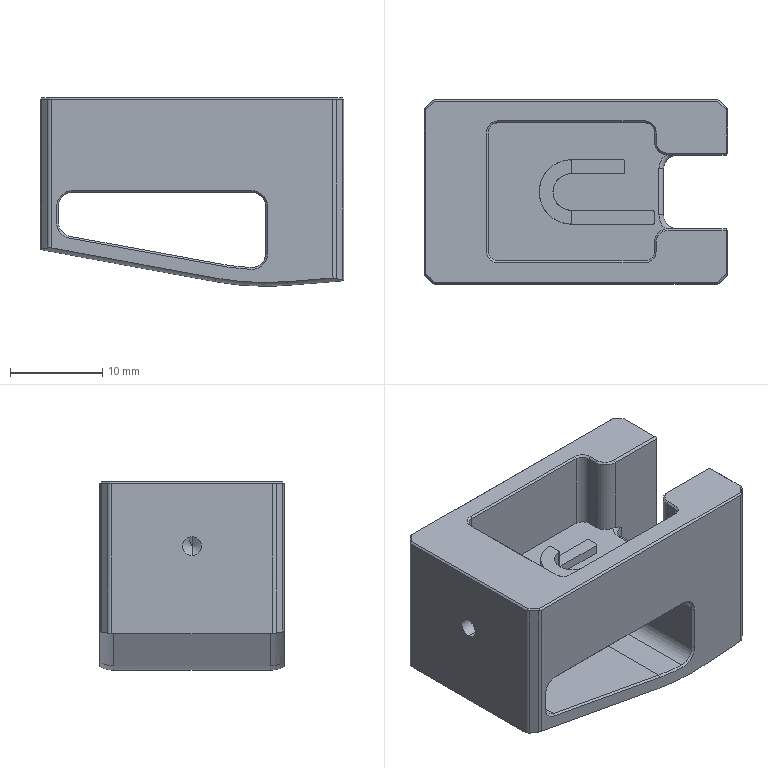NC program | NX | posted with a generic post | part box 33 x 20 x 20.478 mm
Lines 1 to 1476 of 8500:
N10 G17 G21 G94 G90
(FLOOR_WALL , TOOL : D80)
N12 T19 M6
N14 G54
N16 G17 G0 G90 X-64.5 Y0. B0. C0. S6500 M3
N18 G43 Z13. H19
N20 Z3.
N22 G94 G1 Z0. F1500.
N24 X-61.5
N26 X61.5
N28 X64.5
N30 Z3.
N32 G0 Z13.
N34 M5
(ADAPTIVE_MILLING , TOOL : D10)
N36 T15 M6
N38 G54
N40 G17 G0 G90 X-29.197 Y-0.049 B0. C0. S9500 M3
N42 G43 Z11. H15
N44 Z-17.478
N46 G94 G1 Z-20.478 F1000.
N48 X-27.84 Y-0.579 F3000.
N50 G3 X-26.55 Y-0.049 R1.015
N52 X-25.906 Y3.11 R9.424
N54 X-25.693 Y12.706 R184.544
N56 G2 X-22.784 Y17.042 R6.041
N58 X-17.015 Y18.852 R13.38
N60 X-8.025 Y19.178 R88.847
N62 G1 X-6.225 Y19.184
N64 X-3.525 Y19.188
N66 X2.075 Y19.19
N68 X18.775
N70 X18.875 Y19.189
N72 X18.975 Y19.186
N74 G2 X23.412 Y16.453 R5.88
N76 X25.313 Y10.821 R12.745
N78 X25.672 Y2.634 R73.061
N80 X25.665 Y-12.765 R826.306
N82 X22.794 Y-17.018 R6.043
N84 X17.429 Y-18.797 R12.91
N86 X8.943 Y-19.173 R72.366
N88 G1 X7.543 Y-19.18
N90 X5.643 Y-19.185
N92 X2.543 Y-19.189
N94 X-5.657 Y-19.19
N96 X-18.757
N98 X-18.857 Y-19.189
N100 G2 X-23.227 Y-16.711 R5.739
N102 X-25.255 Y-11.235 R12.019
N104 X-25.571 Y-1.555 R52.678
N106 G3 X-24.923 Y10.121 R113.262
N108 G2 X-21.008 Y16.066 R7.723
N110 X-14.843 Y17.969 R15.574
N112 X-5.557 Y18.363 R84.404
N114 G1 X-4.057 Y18.37
N116 X-2.057 Y18.376
N118 X1.043 Y18.38
N120 X8.043 Y18.381
N122 X16.043 Y18.382
N124 X16.143 Y18.381
N126 G2 X22.423 Y14.693 R7.557
N128 X24.435 Y8.568 R14.865
N130 X24.862 Y-0.917 R80.933
N132 X24.843 Y-10.316 R246.554
N134 X20.874 Y-16.119 R7.736
N136 X14.498 Y-18.009 R16.025
N138 X4.809 Y-18.367 R97.281
N140 G1 X3.209 Y-18.373
N142 X0.909 Y-18.378
N144 X-3.191 Y-18.381
N146 X-15.991 Y-18.382
N148 X-16.191 Y-18.38
N150 X-16.391 Y-18.373
N152 G2 X-22.556 Y-14.484 R7.647
N154 X-24.481 Y-8.223 R15.541
N156 X-24.519 Y0.46 R41.857
N158 G3 X-24.138 Y8.349 R857.805
N160 G2 X-19.144 Y15.38 R8.958
N162 X-12.327 Y17.203 R18.779
N164 X-2.337 Y17.556 R111.284
N166 X14.563 Y17.545 R890.638
N168 X21.801 Y12.722 R8.805
N170 X23.698 Y5.825 R18.339
N172 X24.062 Y-5.465 R122.093
N174 X23.845 Y-9.449 R18.233
N176 X18.864 Y-15.488 R9.011
N178 X12.221 Y-17.21 R19.143
N180 X1.331 Y-17.561 R120.966
N182 X-14.568 Y-17.544 R863.034
N184 X-21.805 Y-12.718 R8.797
N186 X-23.724 Y-5.018 R18.167
N188 X-23.56 Y3.077 R99.096
N190 X-23.222 Y7.659 R30.846
N192 X-17.67 Y14.575 R9.873
N194 X-10.537 Y16.389 R20.72
N196 X0.553 Y16.75 R125.976
N198 X12.853 Y16.726 R517.693
N200 X20.669 Y11.829 R9.524
N202 X22.219 Y7.985 R12.151
N204 X23.154 Y-0.347 R39.823
N206 X23.165 Y-6.844 R65.853
N208 X18.349 Y-14.153 R9.47
N210 X14.968 Y-15.59 R11.098
N212 X7.053 Y-16.624 R34.899
N214 X-12.745 Y-16.731 R554.895
N216 X-20.659 Y-11.841 R9.502
N218 X-22.178 Y-8.076 R11.391
N220 X-22.815 Y-0.424 R30.38
N222 X-22.52 Y5.764 R52.429
N224 X-21.597 Y8.818 R12.776
N226 X-20.808 Y11.647 R6.481
N228 X-18.029 Y14.376 R9.736
N230 X-15.327 Y15.096 R6.531
N232 X0.91 Y15.934 R136.055
N234 X11.409 Y15.9 R258.588
N236 X14.907 Y15.115 R12.167
N238 X16.806 Y14.883 R27.804
N240 X19.277 Y13.435 R6.592
N242 X20.711 Y11.773 R10.839
N244 G1 X20.808 Y11.647
N246 X20.876 Y11.529
N248 G2 X21.596 Y8.827 R6.531
N250 X22.374 Y-4.51 R121.46
N252 X21.618 Y-8.318 R11.799
N254 X21.383 Y-10.306 R19.905
N256 X19.935 Y-12.777 R6.592
N258 X18.273 Y-14.211 R10.839
N260 G3 X19.308 Y-15.909 R1.
N262 G1 X19.425 Y-15.854
N264 X21.234 Y-15.002 Z-20.378
N266 X22.493 Y-14.409
N268 X22.639 Y-14.319
N270 X22.773 Y-14.211
N272 X23.379 Y-13.588
N274 G3 X23.822 Y-12.725 R2.463
N276 X25.265 Y-5.267 R39.856
N278 G1 X25.37 Y-3.775
N280 X25.419 Y-2.28
N282 X25.497 Y6.509
N284 G3 X25.26 Y7.164 R1.032
N286 G1 X24.116 Y8.515
N288 X23.69 Y9.027 Z-20.412
N290 X23.245 Y9.522 Z-20.445
N292 G3 X22.634 Y9.758 Z-20.478 R1.04
N294 X21.6 Y8.759 R1.004
N296 G2 X21.535 Y1.067 R447.921
N298 X21.519 Y-3.583 R98.353
N300 G1 X21.596 Y-4.166
N302 X21.6 Y-4.234
N304 Y-8.534
N306 G3 X22.702 Y-9.632 R1.1
N308 X23.8 Y-8.533 R1.1
N310 G1 X23.786 Y4.024
N312 G3 X21.596 Y4.166 R1.1
N314 G2 X21.143 Y1.748 R17.605
N316 G3 X20.89 Y-1.537 R20.735
N318 G1 X20.913 Y-1.634
N320 X20.918 Y-1.67
N322 X20.943 Y-1.714
N324 X21.4 Y-2.816
N326 X21.435 Y-2.948
N328 X21.527 Y-3.642
N330 G3 X23.717 Y-3.461 R1.1
N332 G1 X23.516 Y2.433
N334 G3 X21.4 Y2.816 R1.1
N336 X20.425 Y-0.517 R9.925
N338 X20.875 Y-1.595 R1.48
N340 G1 X20.925 Y-1.682
N342 G3 X22.977 Y-1.141 R1.101
N344 G1 X22.996 Y1.155
N346 G3 X20.943 Y1.714 R1.101
N348 X20.145 Y-0.426 R3.301
N350 X20.619 Y-1.262 R1.968
N352 X22.586 Y-0.7 R1.101
N354 G1 X22.668 Y0.067
N356 X22.724 Y0.836
N358 G3 X20.753 Y1.437 R1.101
N360 X19.968 Y0.068 R3.065
N362 X20.324 Y-0.877 R1.267
N364 X22.281 Y-0.024 R1.101
N366 G1 X22.221 Y0.325
N368 X22.104 Y0.659
N370 G3 X20.266 Y0.802 R1.102
N372 X20.126 Y-0.615 R1.104
N374 G2 X21.435 Y-2.948 R5.91
N376 G1 X21.6 Y-4.234
N378 X21.596 Y-8.827
N380 G2 X20.808 Y-11.647 R6.449
N382 X18.029 Y-14.376 R9.847
N384 X15.327 Y-15.096 R6.531
N386 X-0.51 Y-15.932 R134.597
N388 X-11.409 Y-15.899 R272.221
N390 X-14.908 Y-15.115 R12.161
N392 X-16.806 Y-14.883 R28.628
N394 X-19.277 Y-13.435 R6.592
N396 X-20.711 Y-11.773 R10.839
N398 G3 X-22.409 Y-12.808 R1.
N400 G1 X-22.354 Y-12.925
N402 X-21.502 Y-14.734 Z-20.378
N404 X-20.909 Y-15.993
N406 X-20.819 Y-16.139
N408 X-20.711 Y-16.273
N410 X-20.088 Y-16.878
N412 G3 X-19.222 Y-17.311 R2.374
N414 G1 X-15.893 Y-18.146
N416 G3 X-9.41 Y-18.924 R30.044
N418 G1 X13.009 Y-18.997
N420 G3 X13.657 Y-18.761 R1.033
N422 G1 X15.013 Y-17.616
N424 X15.525 Y-17.19 Z-20.412
N426 X16.022 Y-16.746 Z-20.445
N428 G3 X16.258 Y-16.135 Z-20.478 R1.04
N430 X15.259 Y-15.1 R1.004
N432 G1 X-15.041
N434 G2 X-18.147 Y-14.308 R6.417
N436 X-20.876 Y-11.529 R9.847
N438 X-21.6 Y-8.759 R6.592
N440 X-21.824 Y3.627 R80.534
N442 G1 X-21.803 Y3.825
N444 X-21.779 Y4.024
N446 X-21.752 Y4.222
N448 X-21.738 Y4.321
N450 X-21.707 Y4.519
N452 X-21.655 Y4.814
N454 X-21.619 Y5.011
N456 X-21.603 Y5.11
N458 X-21.6 Y5.134
N460 Y8.759
N462 X-21.596 Y8.827
N464 G3 X-23.793 Y8.899 R-1.1
N466 G1 X-23.8 Y-8.758
N468 G3 X-22.699 Y-9.857 R1.1
N470 X-21.6 Y-8.759 R1.1
N472 G1 Y5.141
N474 X-21.596 Y8.827
N476 G2 X-20.808 Y11.647 R6.449
N478 X-18.029 Y14.376 R9.847
N480 G1 X-16.806 Y14.883
N482 X-16.674 Y14.918
N484 X-15.259 Y15.1
N486 X15.041
N488 G3 X16.011 Y15.828 R1.017
N490 G1 X16.487 Y17.463
N492 Z-17.478
N494 G0 Z11.
N496 M5
(ZLEVEL_PROFILE , TOOL : D6)
N498 T12 M6
N500 G54
N502 G17 G0 G90 X19.81 Y1.615 B0. C0. S9500 M3
N504 G43 Z30. H12
N506 Z0.001
N508 G94 G1 Z-0.499 F1800.
N510 X18.903 Y1.906
N512 G3 X18.317 Y1.779 R0.6
N514 G2 X16.3 Y1. R3.
N516 G1 X12.5
N518 Y-1.
N520 X16.3
N522 G2 X18.317 Y-1.779 R3.
N524 G3 X18.903 Y-1.906 R0.6
N526 G1 X19.81 Y-1.615
N528 Z0.001
N530 G0 Y1.615 Z-0.499
N532 G1 Z-0.999
N534 X18.903 Y1.906
N536 G3 X18.317 Y1.779 R0.6
N538 G2 X16.3 Y1. R3.
N540 G1 X12.5
N542 Y-1.
N544 X16.3
N546 G2 X18.317 Y-1.779 R3.
N548 G3 X18.903 Y-1.906 R0.6
N550 G1 X19.81 Y-1.615
N552 Z-0.499
N554 G0 Y1.615 Z-0.998
N556 G1 Z-1.498
N558 X18.903 Y1.906
N560 G3 X18.317 Y1.779 R0.6
N562 G2 X16.3 Y1. R3.
N564 G1 X12.5
N566 Y-1.
N568 X16.3
N570 G2 X18.317 Y-1.779 R3.
N572 G3 X18.903 Y-1.906 R0.6
N574 G1 X19.81 Y-1.615
N576 Z-0.998
N578 G0 Y1.615 Z-1.498
N580 G1 Z-1.998
N582 X18.903 Y1.906
N584 G3 X18.317 Y1.779 R0.6
N586 G2 X16.3 Y1. R3.
N588 G1 X12.5
N590 Y-1.
N592 X16.3
N594 G2 X18.317 Y-1.779 R3.
N596 G3 X18.903 Y-1.906 R0.6
N598 G1 X19.81 Y-1.615
N600 Z-1.498
N602 G0 Y1.615 Z-1.997
N604 G1 Z-2.497
N606 X18.903 Y1.906
N608 G3 X18.317 Y1.779 R0.6
N610 G2 X16.3 Y1. R3.
N612 G1 X12.5
N614 Y-1.
N616 X16.3
N618 G2 X18.317 Y-1.779 R3.
N620 G3 X18.903 Y-1.906 R0.6
N622 G1 X19.81 Y-1.615
N624 Z-1.997
N626 G0 Y1.615 Z-2.497
N628 G1 Z-2.997
N630 X18.903 Y1.906
N632 G3 X18.317 Y1.779 R0.6
N634 G2 X16.3 Y1. R3.
N636 G1 X12.5
N638 Y-1.
N640 X16.3
N642 G2 X18.317 Y-1.779 R3.
N644 G3 X18.903 Y-1.906 R0.6
N646 G1 X19.81 Y-1.615
N648 Z-2.497
N650 G0 Y1.615 Z-2.996
N652 G1 Z-3.496
N654 X18.903 Y1.906
N656 G3 X18.317 Y1.779 R0.6
N658 G2 X16.3 Y1. R3.
N660 G1 X12.5
N662 Y-1.
N664 X16.3
N666 G2 X18.317 Y-1.779 R3.
N668 G3 X18.903 Y-1.906 R0.6
N670 G1 X19.81 Y-1.615
N672 Z-2.996
N674 G0 Y1.615 Z-3.496
N676 G1 Z-3.996
N678 X18.903 Y1.906
N680 G3 X18.317 Y1.779 R0.6
N682 G2 X16.3 Y1. R3.
N684 G1 X12.5
N686 Y-1.
N688 X16.3
N690 G2 X18.317 Y-1.779 R3.
N692 G3 X18.903 Y-1.906 R0.6
N694 G1 X19.81 Y-1.615
N696 Z-3.496
N698 G0 Y1.615 Z-3.995
N700 G1 Z-4.495
N702 X18.903 Y1.906
N704 G3 X18.317 Y1.779 R0.6
N706 G2 X16.3 Y1. R3.
N708 G1 X12.5
N710 Y-1.
N712 X16.3
N714 G2 X18.317 Y-1.779 R3.
N716 G3 X18.903 Y-1.906 R0.6
N718 G1 X19.81 Y-1.615
N720 Z-3.995
N722 G0 Y1.615 Z-4.495
N724 G1 Z-4.995
N726 X18.903 Y1.906
N728 G3 X18.317 Y1.779 R0.6
N730 G2 X16.3 Y1. R3.
N732 G1 X12.5
N734 Y-1.
N736 X16.3
N738 G2 X18.317 Y-1.779 R3.
N740 G3 X18.903 Y-1.906 R0.6
N742 G1 X19.81 Y-1.615
N744 Z-4.495
N746 G0 Y1.615 Z-4.994
N748 G1 Z-5.494
N750 X18.903 Y1.906
N752 G3 X18.317 Y1.779 R0.6
N754 G2 X16.3 Y1. R3.
N756 G1 X12.5
N758 Y-1.
N760 X16.3
N762 G2 X18.317 Y-1.779 R3.
N764 G3 X18.903 Y-1.906 R0.6
N766 G1 X19.81 Y-1.615
N768 Z-4.994
N770 G0 Y1.615 Z-5.494
N772 G1 Z-5.994
N774 X18.903 Y1.906
N776 G3 X18.317 Y1.779 R0.6
N778 G2 X16.3 Y1. R3.
N780 G1 X12.5
N782 Y-1.
N784 X16.3
N786 G2 X18.317 Y-1.779 R3.
N788 G3 X18.903 Y-1.906 R0.6
N790 G1 X19.81 Y-1.615
N792 Z-5.494
N794 G0 Y1.615 Z-5.993
N796 G1 Z-6.493
N798 X18.903 Y1.906
N800 G3 X18.317 Y1.779 R0.6
N802 G2 X16.3 Y1. R3.
N804 G1 X12.5
N806 Y-1.
N808 X16.3
N810 G2 X18.317 Y-1.779 R3.
N812 G3 X18.903 Y-1.906 R0.6
N814 G1 X19.81 Y-1.615
N816 Z-5.993
N818 G0 Y1.615 Z-6.493
N820 G1 Z-6.993
N822 X18.903 Y1.906
N824 G3 X18.317 Y1.779 R0.6
N826 G2 X16.3 Y1. R3.
N828 G1 X12.5
N830 Y-1.
N832 X16.3
N834 G2 X18.317 Y-1.779 R3.
N836 G3 X18.903 Y-1.906 R0.6
N838 G1 X19.81 Y-1.615
N840 Z-6.493
N842 G0 Y1.615 Z-6.992
N844 G1 Z-7.492
N846 X18.903 Y1.906
N848 G3 X18.317 Y1.779 R0.6
N850 G2 X16.3 Y1. R3.
N852 G1 X12.5
N854 Y-1.
N856 X16.3
N858 G2 X18.317 Y-1.779 R3.
N860 G3 X18.903 Y-1.906 R0.6
N862 G1 X19.81 Y-1.615
N864 Z-6.992
N866 G0 Y1.615 Z-7.492
N868 G1 Z-7.992
N870 X18.903 Y1.906
N872 G3 X18.317 Y1.779 R0.6
N874 G2 X16.3 Y1. R3.
N876 G1 X12.5
N878 Y-1.
N880 X16.3
N882 G2 X18.317 Y-1.779 R3.
N884 G3 X18.903 Y-1.906 R0.6
N886 G1 X19.81 Y-1.615
N888 Z-7.492
N890 G0 Y1.615 Z-7.991
N892 G1 Z-8.491
N894 X18.903 Y1.906
N896 G3 X18.317 Y1.779 R0.6
N898 G2 X16.3 Y1. R3.
N900 G1 X12.5
N902 Y-1.
N904 X16.3
N906 G2 X18.317 Y-1.779 R3.
N908 G3 X18.903 Y-1.906 R0.6
N910 G1 X19.81 Y-1.615
N912 Z-7.991
N914 G0 Y1.615 Z-8.49
N916 G1 Z-8.99
N918 X18.903 Y1.906
N920 G3 X18.317 Y1.779 R0.6
N922 G2 X16.3 Y1. R3.
N924 G1 X12.5
N926 Y-1.
N928 X16.3
N930 G2 X18.317 Y-1.779 R3.
N932 G3 X18.903 Y-1.906 R0.6
N934 G1 X19.81 Y-1.615
N936 Z-8.49
N938 G0 Y1.615 Z-8.99
N940 G1 Z-9.49
N942 X18.903 Y1.906
N944 G3 X18.317 Y1.779 R0.6
N946 G2 X16.3 Y1. R3.
N948 G1 X12.5
N950 Y-1.
N952 X16.3
N954 G2 X18.317 Y-1.779 R3.
N956 G3 X18.903 Y-1.906 R0.6
N958 G1 X19.81 Y-1.615
N960 Z-8.99
N962 G0 Y1.615 Z-9.489
N964 G1 Z-9.989
N966 X18.903 Y1.906
N968 G3 X18.317 Y1.779 R0.6
N970 G2 X16.3 Y1. R3.
N972 G1 X12.5
N974 Y-1.
N976 X16.3
N978 G2 X18.317 Y-1.779 R3.
N980 G3 X18.903 Y-1.906 R0.6
N982 G1 X19.81 Y-1.615
N984 Z-9.489
N986 G0 Y1.615 Z-9.989
N988 G1 Z-10.489
N990 X18.903 Y1.906
N992 G3 X18.317 Y1.779 R0.6
N994 G2 X16.3 Y1. R3.
N996 G1 X12.5
N998 Y-1.
N1000 X16.3
N1002 G2 X18.317 Y-1.779 R3.
N1004 G3 X18.903 Y-1.906 R0.6
N1006 G1 X19.81 Y-1.615
N1008 Z-9.989
N1010 G0 Y1.615 Z-10.488
N1012 G1 Z-10.988
N1014 X18.903 Y1.906
N1016 G3 X18.317 Y1.779 R0.6
N1018 G2 X16.3 Y1. R3.
N1020 G1 X12.5
N1022 Y-1.
N1024 X16.3
N1026 G2 X18.317 Y-1.779 R3.
N1028 G3 X18.903 Y-1.906 R0.6
N1030 G1 X19.81 Y-1.615
N1032 Z-10.488
N1034 G0 Y1.615 Z-10.988
N1036 G1 Z-11.488
N1038 X18.903 Y1.906
N1040 G3 X18.317 Y1.779 R0.6
N1042 G2 X16.3 Y1. R3.
N1044 G1 X12.5
N1046 Y-1.
N1048 X16.3
N1050 G2 X18.317 Y-1.779 R3.
N1052 G3 X18.903 Y-1.906 R0.6
N1054 G1 X19.81 Y-1.615
N1056 Z-10.988
N1058 G0 Y1.615 Z-11.487
N1060 G1 Z-11.987
N1062 X18.903 Y1.906
N1064 G3 X18.317 Y1.779 R0.6
N1066 G2 X16.3 Y1. R3.
N1068 G1 X12.5
N1070 Y-1.
N1072 X16.3
N1074 G2 X18.317 Y-1.779 R3.
N1076 G3 X18.903 Y-1.906 R0.6
N1078 G1 X19.81 Y-1.615
N1080 Z-11.487
N1082 G0 Y1.615 Z-11.987
N1084 G1 Z-12.487
N1086 X18.903 Y1.906
N1088 G3 X18.317 Y1.779 R0.6
N1090 G2 X16.3 Y1. R3.
N1092 G1 X12.5
N1094 Y-1.
N1096 X16.3
N1098 G2 X18.317 Y-1.779 R3.
N1100 G3 X18.903 Y-1.906 R0.6
N1102 G1 X19.81 Y-1.615
N1104 Z-11.987
N1106 G0 Y1.615 Z-12.486
N1108 G1 Z-12.986
N1110 X18.903 Y1.906
N1112 G3 X18.317 Y1.779 R0.6
N1114 G2 X16.3 Y1. R3.
N1116 G1 X12.5
N1118 Y-1.
N1120 X16.3
N1122 G2 X18.317 Y-1.779 R3.
N1124 G3 X18.903 Y-1.906 R0.6
N1126 G1 X19.81 Y-1.615
N1128 Z-12.486
N1130 G0 Y1.615 Z-12.986
N1132 G1 Z-13.486
N1134 X18.903 Y1.906
N1136 G3 X18.317 Y1.779 R0.6
N1138 G2 X16.3 Y1. R3.
N1140 G1 X12.5
N1142 Y-1.
N1144 X16.3
N1146 G2 X18.317 Y-1.779 R3.
N1148 G3 X18.903 Y-1.906 R0.6
N1150 G1 X19.81 Y-1.615
N1152 Z-12.986
N1154 G0 Y1.615 Z-13.485
N1156 G1 Z-13.985
N1158 X18.903 Y1.906
N1160 G3 X18.317 Y1.779 R0.6
N1162 G2 X16.3 Y1. R3.
N1164 G1 X12.5
N1166 Y-1.
N1168 X16.3
N1170 G2 X18.317 Y-1.779 R3.
N1172 G3 X18.903 Y-1.906 R0.6
N1174 G1 X19.81 Y-1.615
N1176 Z-13.485
N1178 G0 Y1.615 Z-13.985
N1180 G1 Z-14.485
N1182 X18.903 Y1.906
N1184 G3 X18.317 Y1.779 R0.6
N1186 G2 X16.3 Y1. R3.
N1188 G1 X12.5
N1190 Y-1.
N1192 X16.3
N1194 G2 X18.317 Y-1.779 R3.
N1196 G3 X18.903 Y-1.906 R0.6
N1198 G1 X19.81 Y-1.615
N1200 Z-13.985
N1202 G0 Y1.615 Z-14.484
N1204 G1 Z-14.984
N1206 X18.903 Y1.906
N1208 G3 X18.317 Y1.779 R0.6
N1210 G2 X16.3 Y1. R3.
N1212 G1 X12.5
N1214 Y-1.
N1216 X16.3
N1218 G2 X18.317 Y-1.779 R3.
N1220 G3 X18.903 Y-1.906 R0.6
N1222 G1 X19.81 Y-1.615
N1224 Z-14.484
N1226 G0 Y1.615 Z-14.984
N1228 G1 Z-15.484
N1230 X18.903 Y1.906
N1232 G3 X18.317 Y1.779 R0.6
N1234 G2 X16.3 Y1. R3.
N1236 G1 X12.5
N1238 Y-1.
N1240 X16.3
N1242 G2 X18.317 Y-1.779 R3.
N1244 G3 X18.903 Y-1.906 R0.6
N1246 G1 X19.81 Y-1.615
N1248 Z-14.984
N1250 G0 Y1.615 Z-15.483
N1252 G1 Z-15.983
N1254 X18.903 Y1.906
N1256 G3 X18.317 Y1.779 R0.6
N1258 G2 X16.3 Y1. R3.
N1260 G1 X12.5
N1262 Y-1.
N1264 X16.3
N1266 G2 X18.317 Y-1.779 R3.
N1268 G3 X18.903 Y-1.906 R0.6
N1270 G1 X19.81 Y-1.615
N1272 Z-15.483
N1274 G0 Y1.615 Z-15.983
N1276 G1 Z-16.483
N1278 X18.903 Y1.906
N1280 G3 X18.317 Y1.779 R0.6
N1282 G2 X16.3 Y1. R3.
N1284 G1 X12.5
N1286 Y-1.
N1288 X16.3
N1290 G2 X18.317 Y-1.779 R3.
N1292 G3 X18.903 Y-1.906 R0.6
N1294 G1 X19.81 Y-1.615
N1296 Z-15.983
N1298 G0 Y1.615 Z-16.482
N1300 G1 Z-16.982
N1302 X18.903 Y1.906
N1304 G3 X18.317 Y1.779 R0.6
N1306 G2 X16.3 Y1. R3.
N1308 G1 X12.5
N1310 Y-1.
N1312 X16.3
N1314 G2 X18.317 Y-1.779 R3.
N1316 G3 X18.903 Y-1.906 R0.6
N1318 G1 X19.81 Y-1.615
N1320 Z-16.482
N1322 G0 Y1.615 Z-16.981
N1324 G1 Z-17.481
N1326 X18.903 Y1.906
N1328 G3 X18.317 Y1.779 R0.6
N1330 G2 X16.3 Y1. R3.
N1332 G1 X12.5
N1334 Y-1.
N1336 X16.3
N1338 G2 X18.317 Y-1.779 R3.
N1340 G3 X18.903 Y-1.906 R0.6
N1342 G1 X19.81 Y-1.615
N1344 Z-16.981
N1346 G0 Y1.615 Z-17.481
N1348 G1 Z-17.981
N1350 X18.903 Y1.906
N1352 G3 X18.317 Y1.779 R0.6
N1354 G2 X16.3 Y1. R3.
N1356 G1 X12.5
N1358 Y-1.
N1360 X16.3
N1362 G2 X18.317 Y-1.779 R3.
N1364 G3 X18.903 Y-1.906 R0.6
N1366 G1 X19.81 Y-1.615
N1368 Z-17.481
N1370 G0 Y1.615 Z-17.98
N1372 G1 Z-18.48
N1374 X18.903 Y1.906
N1376 G3 X18.317 Y1.779 R0.6
N1378 G2 X16.3 Y1. R3.
N1380 G1 X12.5
N1382 Y-1.
N1384 X16.3
N1386 G2 X18.317 Y-1.779 R3.
N1388 G3 X18.903 Y-1.906 R0.6
N1390 G1 X19.81 Y-1.615
N1392 Z-17.98
N1394 G0 Y1.615 Z-18.48
N1396 G1 Z-18.98
N1398 X18.903 Y1.906
N1400 G3 X18.317 Y1.779 R0.6
N1402 G2 X16.3 Y1. R3.
N1404 G1 X12.5
N1406 Y-1.
N1408 X16.3
N1410 G2 X18.317 Y-1.779 R3.
N1412 G3 X18.903 Y-1.906 R0.6
N1414 G1 X19.81 Y-1.615
N1416 Z-18.48
N1418 G0 Y1.615 Z-18.979
N1420 G1 Z-19.479
N1422 X18.903 Y1.906
N1424 G3 X18.317 Y1.779 R0.6
N1426 G2 X16.3 Y1. R3.
N1428 G1 X12.5
N1430 Y-1.
N1432 X16.3
N1434 G2 X18.317 Y-1.779 R3.
N1436 G3 X18.903 Y-1.906 R0.6
N1438 G1 X19.81 Y-1.615
N1440 Z-18.979
N1442 G0 Y1.615 Z-19.479
N1444 G1 Z-19.979
N1446 X18.903 Y1.906
N1448 G3 X18.317 Y1.779 R0.6
N1450 G2 X16.3 Y1. R3.
N1452 G1 X12.5
N1454 Y-1.
N1456 X16.3
N1458 G2 X18.317 Y-1.779 R3.
N1460 G3 X18.903 Y-1.906 R0.6
N1462 G1 X19.81 Y-1.615
N1464 Z-19.479
N1466 G0 Y1.615 Z-19.978
N1468 G1 Z-20.478
N1470 X18.903 Y1.906
N1472 G3 X18.317 Y1.779 R0.6
N1474 G2 X16.3 Y1. R3.
N1476 G1 X12.5
N1478 Y-1.
N1480 X16.3
N1482 G2 X18.317 Y-1.779 R3.
N1484 G3 X18.903 Y-1.906 R0.6
N1486 G1 X19.81 Y-1.615
N1488 Z-19.978
N1490 G0 Z30.
(CAVITY_MILL , TOOL : D6)
N1492 X3.531 Y-0.442
N1494 Z11.
N1496 Z1.
N1498 G1 X3.574 Y-0.38 Z0.996 F1000.
N1500 X3.918 Y0. Z0.969
N1502 X3.574 Y0.38 Z0.942
N1504 X3.281 Y0.8 Z0.915
N1506 X-2.8 Z0.597
N1508 Y-0.8 Z0.513
N1510 X3.281 Z0.194
N1512 X3.574 Y-0.38 Z0.167
N1514 X3.918 Y0. Z0.141
N1516 X3.574 Y0.38 Z0.114
N1518 X3.281 Y0.8 Z0.087
N1520 X-2.8 Z-0.232
N1522 Y-0.8 Z-0.316
N1524 X0.24 Z-0.475
N1526 X3.281 F2500.
N1528 G2 X3.918 Y0. R8.2
N1530 X3.281 Y0.8 R8.2
N1532 G1 X-2.8
N1534 Y-0.8
N1536 X0.24
N1538 Y-4.4
N1540 X5.533
N1542 G2 X10. Y-0.9 R4.6
N1544 G1 X12.659
N1546 X12.658 Y0.9
N1548 X10.
N1550 G2 X5.533 Y4.4 R4.6
N1552 G1 X-6.4
N1554 Y-4.4
N1556 X0.24
N1558 G3 X1.106 Y-3.9 R1.
N1560 G1 Z1.025
N1562 G0 Z11.
N1564 X-2.8 Y0.363
N1566 Z0.525
N1568 G1 Y-0.8 Z0.464 F1000.
N1570 X3.281 Z0.145
N1572 X3.574 Y-0.38 Z0.119
N1574 X3.918 Y0. Z0.092
N1576 X3.574 Y0.38 Z0.065
N1578 X3.281 Y0.8 Z0.038
N1580 X-2.8 Z-0.281
N1582 Y-0.8 Z-0.365
N1584 X3.281 Z-0.683
N1586 X3.574 Y-0.38 Z-0.71
N1588 X3.918 Y0. Z-0.737
N1590 X3.574 Y0.38 Z-0.764
N1592 X3.281 Y0.8 Z-0.791
N1594 X0.24 Z-0.95
N1596 X-2.8 F2500.
N1598 Y-0.8
N1600 X3.281
N1602 G2 X3.918 Y0. R8.2
N1604 X3.281 Y0.8 R8.2
N1606 G1 X0.24
N1608 Y4.4
N1610 X-6.4
N1612 Y-4.4
N1614 X5.533
N1616 G2 X10. Y-0.9 R4.6
N1618 G1 X12.659
N1620 X12.658 Y0.9
N1622 X10.
N1624 G2 X5.533 Y4.4 R4.6
N1626 G1 X0.24
N1628 G3 X-0.626 Y3.9 R1.
N1630 G1 Z0.55
N1632 G0 Z11.
N1634 X-2.8 Y0.363
N1636 Z0.05
N1638 G1 Y-0.8 Z-0.011 F1000.
N1640 X3.281 Z-0.33
N1642 X3.574 Y-0.38 Z-0.356
N1644 X3.918 Y0. Z-0.383
N1646 X3.574 Y0.38 Z-0.41
N1648 X3.281 Y0.8 Z-0.437
N1650 X-2.8 Z-0.756
N1652 Y-0.8 Z-0.84
N1654 X3.281 Z-1.158
N1656 X3.574 Y-0.38 Z-1.185
N1658 X3.918 Y0. Z-1.212
N1660 X3.574 Y0.38 Z-1.239
N1662 X3.281 Y0.8 Z-1.266
N1664 X0.24 Z-1.425
N1666 X-2.8 F2500.
N1668 Y-0.8
N1670 X3.281
N1672 G2 X3.918 Y0. R8.2
N1674 X3.281 Y0.8 R8.2
N1676 G1 X0.24
N1678 Y4.4
N1680 X-6.4
N1682 Y-4.4
N1684 X5.533
N1686 G2 X10. Y-0.9 R4.6
N1688 G1 X12.659
N1690 X12.658 Y0.9
N1692 X10.
N1694 G2 X5.533 Y4.4 R4.6
N1696 G1 X0.24
N1698 G3 X-0.626 Y3.9 R1.
N1700 G1 Z0.075
N1702 G0 X3.531 Y-0.442 Z-0.425
N1704 G1 X3.574 Y-0.38 Z-0.429 F1000.
N1706 X3.918 Y0. Z-0.456
N1708 X3.574 Y0.38 Z-0.483
N1710 X3.281 Y0.8 Z-0.51
N1712 X-2.8 Z-0.828
N1714 Y-0.8 Z-0.912
N1716 X3.281 Z-1.231
N1718 X3.574 Y-0.38 Z-1.258
N1720 X3.918 Y0. Z-1.284
N1722 X3.574 Y0.38 Z-1.311
N1724 X3.281 Y0.8 Z-1.338
N1726 X-2.8 Z-1.657
N1728 Y-0.8 Z-1.741
N1730 X0.24 Z-1.9
N1732 X3.281 F2500.
N1734 G2 X3.918 Y0. R8.2
N1736 X3.281 Y0.8 R8.2
N1738 G1 X-2.8
N1740 Y-0.8
N1742 X0.24
N1744 Y-4.4
N1746 X5.533
N1748 G2 X10. Y-0.9 R4.6
N1750 G1 X12.659
N1752 X12.658 Y0.9
N1754 X10.
N1756 G2 X5.533 Y4.4 R4.6
N1758 G1 X-6.4
N1760 Y-4.4
N1762 X0.24
N1764 G3 X1.106 Y-3.9 R1.
N1766 G1 Z-0.4
N1768 G0 X3.531 Y-0.442 Z-0.9
N1770 G1 X3.574 Y-0.38 Z-0.904 F1000.
N1772 X3.918 Y0. Z-0.931
N1774 X3.574 Y0.38 Z-0.958
N1776 X3.281 Y0.8 Z-0.985
N1778 X-2.8 Z-1.303
N1780 Y-0.8 Z-1.387
N1782 X3.281 Z-1.706
N1784 X3.574 Y-0.38 Z-1.733
N1786 X3.918 Y0. Z-1.759
N1788 X3.574 Y0.38 Z-1.786
N1790 X3.281 Y0.8 Z-1.813
N1792 X-2.8 Z-2.132
N1794 Y-0.8 Z-2.216
N1796 X0.24 Z-2.375
N1798 X3.281 F2500.
N1800 G2 X3.918 Y0. R8.2
N1802 X3.281 Y0.8 R8.2
N1804 G1 X-2.8
N1806 Y-0.8
N1808 X0.24
N1810 Y-4.4
N1812 X5.533
N1814 G2 X10. Y-0.9 R4.6
N1816 G1 X12.659
N1818 X12.658 Y0.9
N1820 X10.
N1822 G2 X5.533 Y4.4 R4.6
N1824 G1 X-6.4
N1826 Y-4.4
N1828 X0.24
N1830 G3 X1.106 Y-3.9 R1.
N1832 G1 Z-0.875
N1834 G0 X-2.8 Y0.363 Z-1.375
N1836 G1 Y-0.8 Z-1.436 F1000.
N1838 X3.281 Z-1.755
N1840 X3.574 Y-0.38 Z-1.781
N1842 X3.918 Y0. Z-1.808
N1844 X3.574 Y0.38 Z-1.835
N1846 X3.281 Y0.8 Z-1.862
N1848 X-2.8 Z-2.181
N1850 Y-0.8 Z-2.265
N1852 X3.281 Z-2.583
N1854 X3.574 Y-0.38 Z-2.61
N1856 X3.918 Y0. Z-2.637
N1858 X3.574 Y0.38 Z-2.664
N1860 X3.281 Y0.8 Z-2.691
N1862 X0.24 Z-2.85
N1864 X-2.8 F2500.
N1866 Y-0.8
N1868 X3.281
N1870 G2 X3.918 Y0. R8.2
N1872 X3.281 Y0.8 R8.2
N1874 G1 X0.24
N1876 Y4.4
N1878 X-6.4
N1880 Y-4.4
N1882 X5.533
N1884 G2 X10. Y-0.9 R4.6
N1886 G1 X12.659
N1888 X12.658 Y0.9
N1890 X10.
N1892 G2 X5.533 Y4.4 R4.6
N1894 G1 X0.24
N1896 G3 X-0.626 Y3.9 R1.
N1898 G1 Z-1.35
N1900 G0 X3.531 Y-0.442 Z-1.85
N1902 G1 X3.574 Y-0.38 Z-1.854 F1000.
N1904 X3.918 Y0. Z-1.881
N1906 X3.574 Y0.38 Z-1.908
N1908 X3.281 Y0.8 Z-1.935
N1910 X-2.8 Z-2.253
N1912 Y-0.8 Z-2.337
N1914 X3.281 Z-2.656
N1916 X3.574 Y-0.38 Z-2.683
N1918 X3.918 Y0. Z-2.709
N1920 X3.574 Y0.38 Z-2.736
N1922 X3.281 Y0.8 Z-2.763
N1924 X-2.8 Z-3.082
N1926 Y-0.8 Z-3.166
N1928 X0.24 Z-3.325
N1930 X3.281 F2500.
N1932 G2 X3.918 Y0. R8.2
N1934 X3.281 Y0.8 R8.2
N1936 G1 X-2.8
N1938 Y-0.8
N1940 X0.24
N1942 Y-4.4
N1944 X5.533
N1946 G2 X10. Y-0.9 R4.6
N1948 G1 X12.659
N1950 X12.658 Y0.9
N1952 X10.
N1954 G2 X5.533 Y4.4 R4.6
N1956 G1 X-6.4
N1958 Y-4.4
N1960 X0.24
N1962 G3 X1.106 Y-3.9 R1.
N1964 G1 Z-1.825
N1966 G0 X-2.8 Y0.363 Z-2.325
N1968 G1 Y-0.8 Z-2.386 F1000.
N1970 X3.281 Z-2.705
N1972 X3.574 Y-0.38 Z-2.731
N1974 X3.918 Y0. Z-2.758
N1976 X3.574 Y0.38 Z-2.785
N1978 X3.281 Y0.8 Z-2.812
N1980 X-2.8 Z-3.131
N1982 Y-0.8 Z-3.215
N1984 X3.281 Z-3.533
N1986 X3.574 Y-0.38 Z-3.56
N1988 X3.918 Y0. Z-3.587
N1990 X3.574 Y0.38 Z-3.614
N1992 X3.281 Y0.8 Z-3.641
N1994 X0.24 Z-3.8
N1996 X-2.8 F2500.
N1998 Y-0.8
N2000 X3.281
N2002 G2 X3.918 Y0. R8.2
N2004 X3.281 Y0.8 R8.2
N2006 G1 X0.24
N2008 Y4.4
N2010 X-6.4
N2012 Y-4.4
N2014 X5.533
N2016 G2 X10. Y-0.9 R4.6
N2018 G1 X12.659
N2020 X12.658 Y0.9
N2022 X10.
N2024 G2 X5.533 Y4.4 R4.6
N2026 G1 X0.24
N2028 G3 X-0.626 Y3.9 R1.
N2030 G1 Z-2.3
N2032 G0 X3.531 Y-0.442 Z-2.8
N2034 G1 X3.574 Y-0.38 Z-2.804 F1000.
N2036 X3.918 Y0. Z-2.831
N2038 X3.574 Y0.38 Z-2.858
N2040 X3.281 Y0.8 Z-2.885
N2042 X-2.8 Z-3.203
N2044 Y-0.8 Z-3.287
N2046 X3.281 Z-3.606
N2048 X3.574 Y-0.38 Z-3.633
N2050 X3.918 Y0. Z-3.659
N2052 X3.574 Y0.38 Z-3.686
N2054 X3.281 Y0.8 Z-3.713
N2056 X-2.8 Z-4.032
N2058 Y-0.8 Z-4.116
N2060 X0.24 Z-4.275
N2062 X3.281 F2500.
N2064 G2 X3.918 Y0. R8.2
N2066 X3.281 Y0.8 R8.2
N2068 G1 X-2.8
N2070 Y-0.8
N2072 X0.24
N2074 Y-4.4
N2076 X5.533
N2078 G2 X10. Y-0.9 R4.6
N2080 G1 X12.659
N2082 X12.658 Y0.9
N2084 X10.
N2086 G2 X5.533 Y4.4 R4.6
N2088 G1 X-6.4
N2090 Y-4.4
N2092 X0.24
N2094 G3 X1.106 Y-3.9 R1.
N2096 G1 Z-2.775
N2098 G0 X3.531 Y-0.442 Z-3.275
N2100 G1 X3.574 Y-0.38 Z-3.279 F1000.
N2102 X3.918 Y0. Z-3.306
N2104 X3.574 Y0.38 Z-3.333
N2106 X3.281 Y0.8 Z-3.36
N2108 X-2.8 Z-3.678
N2110 Y-0.8 Z-3.762
N2112 X3.281 Z-4.081
N2114 X3.574 Y-0.38 Z-4.108
N2116 X3.918 Y0. Z-4.134
N2118 X3.574 Y0.38 Z-4.161
N2120 X3.281 Y0.8 Z-4.188
N2122 X-2.8 Z-4.507
N2124 Y-0.8 Z-4.591
N2126 X0.24 Z-4.75
N2128 X3.281 F2500.
N2130 G2 X3.918 Y0. R8.2
N2132 X3.281 Y0.8 R8.2
N2134 G1 X-2.8
N2136 Y-0.8
N2138 X0.24
N2140 Y-4.4
N2142 X5.533
N2144 G2 X10. Y-0.9 R4.6
N2146 G1 X12.659
N2148 X12.658 Y0.9
N2150 X10.
N2152 G2 X5.533 Y4.4 R4.6
N2154 G1 X-6.4
N2156 Y-4.4
N2158 X0.24
N2160 G3 X1.106 Y-3.9 R1.
N2162 G1 Z-3.25
N2164 G0 X3.531 Y-0.442 Z-3.75
N2166 G1 X3.574 Y-0.38 Z-3.754 F1000.
N2168 X3.918 Y0. Z-3.781
N2170 X3.574 Y0.38 Z-3.808
N2172 X3.281 Y0.8 Z-3.835
N2174 X-2.8 Z-4.153
N2176 Y-0.8 Z-4.237
N2178 X3.281 Z-4.556
N2180 X3.574 Y-0.38 Z-4.583
N2182 X3.918 Y0. Z-4.609
N2184 X3.574 Y0.38 Z-4.636
N2186 X3.281 Y0.8 Z-4.663
N2188 X-2.8 Z-4.982
N2190 Y-0.8 Z-5.066
N2192 X0.24 Z-5.225
N2194 X3.281 F2500.
N2196 G2 X3.918 Y0. R8.2
N2198 X3.281 Y0.8 R8.2
N2200 G1 X-2.8
N2202 Y-0.8
N2204 X0.24
N2206 Y-4.4
N2208 X5.533
N2210 G2 X10. Y-0.9 R4.6
N2212 G1 X12.659
N2214 X12.658 Y0.9
N2216 X10.
N2218 G2 X5.533 Y4.4 R4.6
N2220 G1 X-6.4
N2222 Y-4.4
N2224 X0.24
N2226 G3 X1.106 Y-3.9 R1.
N2228 G1 Z-3.725
N2230 G0 X3.531 Y-0.442 Z-4.225
N2232 G1 X3.574 Y-0.38 Z-4.229 F1000.
N2234 X3.918 Y0. Z-4.256
N2236 X3.574 Y0.38 Z-4.283
N2238 X3.281 Y0.8 Z-4.31
N2240 X-2.8 Z-4.628
N2242 Y-0.8 Z-4.712
N2244 X3.281 Z-5.031
N2246 X3.574 Y-0.38 Z-5.058
N2248 X3.918 Y0. Z-5.084
N2250 X3.574 Y0.38 Z-5.111
N2252 X3.281 Y0.8 Z-5.138
N2254 X-2.8 Z-5.457
N2256 Y-0.8 Z-5.541
N2258 X0.24 Z-5.7
N2260 X3.281 F2500.
N2262 G2 X3.918 Y0. R8.2
N2264 X3.281 Y0.8 R8.2
N2266 G1 X-2.8
N2268 Y-0.8
N2270 X0.24
N2272 Y-4.4
N2274 X5.533
N2276 G2 X10. Y-0.9 R4.6
N2278 G1 X12.659
N2280 X12.658 Y0.9
N2282 X10.
N2284 G2 X5.533 Y4.4 R4.6
N2286 G1 X-6.4
N2288 Y-4.4
N2290 X0.24
N2292 G3 X1.106 Y-3.9 R1.
N2294 G1 Z-4.2
N2296 G0 X2.564 Y3.95 Z-4.7
N2298 G1 X2.6 Y3.74 Z-4.711 F1000.
N2300 Y1.745 Z-4.816
N2302 X2.563 Y1.525 Z-4.827
N2304 X2.269 Y0.683 Z-4.874
N2306 X2.064 Y0.334 Z-4.895
N2308 X1.768 Y0. Z-4.919
N2310 X2.064 Y-0.334 Z-4.942
N2312 X2.269 Y-0.683 Z-4.963
N2314 X2.563 Y-1.525 Z-5.01
N2316 X2.6 Y-1.745 Z-5.022
N2318 Y-3.74 Z-5.126
N2320 X2.559 Y-3.98 Z-5.139
N2322 X2.409 Y-4.4 Z-5.162
N2324 X5.533 Z-5.326
N2326 X5.659 Y-3.889 Z-5.354
N2328 X5.995 Y-3.177 Z-5.395
N2330 X6.446 Y-2.532 Z-5.436
N2332 X6.9 Y-2.1 Z-5.469
N2334 X7.372 Y-1.688 Z-5.502
N2336 X8.374 Y-1.165 Z-5.561
N2338 X9.474 Y-0.9 Z-5.62
N2340 X10. Z-5.648
N2342 X12.659 Y-0.899 Z-5.788
N2344 X12.658 Y0.9 Z-5.882
N2346 X9.474 Z-6.049
N2348 X8.374 Y1.165 Z-6.108
N2350 X7.372 Y1.688 Z-6.167
N2352 X6.901 Y2.101 Z-6.2
N2354 X5.081 Y0.106
N2356 X4.965 Y0.214 F2500.
N2358 G2 X4.886 Y0. R6.
N2360 X4.965 Y-0.214 R6.
N2362 X5.2 Y0. R7.3
N2364 G1 X5.081 Y0.106
N2366 X6.901 Y2.101
N2368 G2 X5.533 Y4.4 R4.6
N2370 G1 X2.409
N2372 G2 X2.6 Y3.294 R3.3
N2374 G1 Y2.191
N2376 G2 X1.768 Y0. R3.3
N2378 X2.6 Y-2.191 R3.3
N2380 G1 Y-3.294
N2382 G2 X2.409 Y-4.4 R3.3
N2384 G1 X5.533
N2386 G2 X10. Y-0.9 R4.6
N2388 G1 X12.659
N2390 X12.658 Y0.9
N2392 X10.
N2394 G2 X6.901 Y2.101 R4.6
N2396 G3 X5.924 Y2.315 R1.
N2398 G1 Z-4.7
N2400 G0 Z11.
N2402 X12.659 Y-0.646
N2404 Z-5.2
N2406 G1 X12.658 Y0.9 Z-5.281 F1000.
N2408 X9.474 Z-5.448
N2410 X8.374 Y1.165 Z-5.507
N2412 X7.372 Y1.688 Z-5.566
N2414 X6.9 Y2.1 Z-5.599
N2416 X6.446 Y2.532 Z-5.632
N2418 X5.995 Y3.177 Z-5.673
N2420 X5.659 Y3.889 Z-5.715
N2422 X5.533 Y4.4 Z-5.742
N2424 X2.409 Z-5.906
N2426 X2.559 Y3.98 Z-5.929
N2428 X2.6 Y3.74 Z-5.942
N2430 Y1.745 Z-6.047
N2432 X2.563 Y1.525 Z-6.058
N2434 X2.269 Y0.683 Z-6.105
N2436 X2.064 Y0.334 Z-6.126
N2438 X1.768 Y0. Z-6.15
N2440 X2.064 Y-0.334 Z-6.173
N2442 X2.269 Y-0.683 Z-6.194
N2444 X2.563 Y-1.525 Z-6.241
N2446 X2.6 Y-1.745 Z-6.253
N2448 Y-3.74 Z-6.357
N2450 X2.559 Y-3.98 Z-6.37
N2452 X2.409 Y-4.4 Z-6.393
N2454 X5.533 Z-6.557
N2456 X5.659 Y-3.889 Z-6.585
N2458 X5.995 Y-3.177 Z-6.626
N2460 X6.446 Y-2.532 Z-6.667
N2462 X6.901 Y-2.101 Z-6.7
N2464 X5.081 Y-0.106
N2466 X5.2 Y0. F2500.
N2468 G2 X4.965 Y0.214 R7.3
N2470 X4.886 Y0. R6.
N2472 X4.965 Y-0.214 R6.
N2474 G1 X5.081 Y-0.106
N2476 X6.901 Y-2.101
N2478 G2 X10. Y-0.9 R4.6
N2480 G1 X12.659
N2482 X12.658 Y0.9
N2484 X10.
N2486 G2 X5.533 Y4.4 R4.6
N2488 G1 X2.409
N2490 G2 X2.6 Y3.294 R3.3
N2492 G1 Y2.191
N2494 G2 X1.768 Y0. R3.3
N2496 X2.6 Y-2.191 R3.3
N2498 G1 Y-3.294
N2500 G2 X2.409 Y-4.4 R3.3
N2502 G1 X5.533
N2504 G2 X6.901 Y-2.101 R4.6
N2506 G3 X7.04 Y-1.883 R0.5
N2508 G1 Z-5.2
N2510 G0 X2.564 Y3.95 Z-5.7
N2512 G1 X2.6 Y3.74 Z-5.711 F1000.
N2514 Y1.745 Z-5.816
N2516 X2.563 Y1.525 Z-5.827
N2518 X2.269 Y0.683 Z-5.874
N2520 X2.064 Y0.334 Z-5.895
N2522 X1.768 Y0. Z-5.919
N2524 X2.064 Y-0.334 Z-5.942
N2526 X2.269 Y-0.683 Z-5.963
N2528 X2.563 Y-1.525 Z-6.01
N2530 X2.6 Y-1.745 Z-6.022
N2532 Y-3.74 Z-6.126
N2534 X2.559 Y-3.98 Z-6.139
N2536 X2.409 Y-4.4 Z-6.162
N2538 X5.533 Z-6.326
N2540 X5.659 Y-3.889 Z-6.354
N2542 X5.995 Y-3.177 Z-6.395
N2544 X6.446 Y-2.532 Z-6.436
N2546 X6.9 Y-2.1 Z-6.469
N2548 X7.372 Y-1.688 Z-6.502
N2550 X8.374 Y-1.165 Z-6.561
N2552 X9.474 Y-0.9 Z-6.62
N2554 X10. Z-6.648
N2556 X12.659 Y-0.899 Z-6.788
N2558 X12.658 Y0.9 Z-6.882
N2560 X9.474 Z-7.049
N2562 X8.374 Y1.165 Z-7.108
N2564 X7.372 Y1.688 Z-7.167
N2566 X6.901 Y2.101 Z-7.2
N2568 X5.081 Y0.106
N2570 X4.965 Y0.214 F2500.
N2572 G2 X4.886 Y0. R6.
N2574 X4.965 Y-0.214 R6.
N2576 X5.2 Y0. R7.3
N2578 G1 X5.081 Y0.106
N2580 X6.901 Y2.101
N2582 G2 X5.533 Y4.4 R4.6
N2584 G1 X2.409
N2586 G2 X2.6 Y3.294 R3.3
N2588 G1 Y2.191
N2590 G2 X1.768 Y0. R3.3
N2592 X2.6 Y-2.191 R3.3
N2594 G1 Y-3.294
N2596 G2 X2.409 Y-4.4 R3.3
N2598 G1 X5.533
N2600 G2 X10. Y-0.9 R4.6
N2602 G1 X12.659
N2604 X12.658 Y0.9
N2606 X10.
N2608 G2 X6.901 Y2.101 R4.6
N2610 G3 X5.924 Y2.315 R1.
N2612 G1 Z-5.7
N2614 G0 Z11.
N2616 X12.659 Y-0.646
N2618 Z-6.2
N2620 G1 X12.658 Y0.9 Z-6.281 F1000.
N2622 X9.474 Z-6.448
N2624 X8.374 Y1.165 Z-6.507
N2626 X7.372 Y1.688 Z-6.566
N2628 X6.9 Y2.1 Z-6.599
N2630 X6.446 Y2.532 Z-6.632
N2632 X5.995 Y3.177 Z-6.673
N2634 X5.659 Y3.889 Z-6.715
N2636 X5.533 Y4.4 Z-6.742
N2638 X2.409 Z-6.906
N2640 X2.559 Y3.98 Z-6.929
N2642 X2.6 Y3.74 Z-6.942
N2644 Y1.745 Z-7.047
N2646 X2.563 Y1.525 Z-7.058
N2648 X2.269 Y0.683 Z-7.105
N2650 X2.064 Y0.334 Z-7.126
N2652 X1.768 Y0. Z-7.15
N2654 X2.064 Y-0.334 Z-7.173
N2656 X2.269 Y-0.683 Z-7.194
N2658 X2.563 Y-1.525 Z-7.241
N2660 X2.6 Y-1.745 Z-7.253
N2662 Y-3.74 Z-7.357
N2664 X2.559 Y-3.98 Z-7.37
N2666 X2.409 Y-4.4 Z-7.393
N2668 X5.533 Z-7.557
N2670 X5.659 Y-3.889 Z-7.585
N2672 X5.995 Y-3.177 Z-7.626
N2674 X6.446 Y-2.532 Z-7.667
N2676 X6.901 Y-2.101 Z-7.7
N2678 X5.081 Y-0.106
N2680 X5.2 Y0. F2500.
N2682 G2 X4.965 Y0.214 R7.3
N2684 X4.886 Y0. R6.
N2686 X4.965 Y-0.214 R6.
N2688 G1 X5.081 Y-0.106
N2690 X6.901 Y-2.101
N2692 G2 X10. Y-0.9 R4.6
N2694 G1 X12.659
N2696 X12.658 Y0.9
N2698 X10.
N2700 G2 X5.533 Y4.4 R4.6
N2702 G1 X2.409
N2704 G2 X2.6 Y3.294 R3.3
N2706 G1 Y2.191
N2708 G2 X1.768 Y0. R3.3
N2710 X2.6 Y-2.191 R3.3
N2712 G1 Y-3.294
N2714 G2 X2.409 Y-4.4 R3.3
N2716 G1 X5.533
N2718 G2 X6.901 Y-2.101 R4.6
N2720 G3 X7.04 Y-1.883 R0.5
N2722 G1 Z-6.2
N2724 G0 X11.268 Y0.9 Z-6.7
N2726 G1 X9.618 Z-6.786 F1000.
N2728 X9.241 Y0.963 Z-6.807
N2730 X9.668 Y0.836 Z-6.83
N2732 X10.514 Y0.287 Z-6.883
N2734 X11.157 Y-0.49 Z-6.936
N2736 X11.333 Y-0.9 Z-6.959
N2738 X12.659 Y-0.899 Z-7.029
N2740 Y-0.007 Z-7.075
N2742 X12.658 Y0.9 Z-7.123
N2744 X9.618 Z-7.282
N2746 X9.241 Y0.963 Z-7.302
N2748 X9.668 Y0.836 Z-7.326
N2750 X10.514 Y0.287 Z-7.378
N2752 X11.157 Y-0.49 Z-7.431
N2754 X11.333 Y-0.9 Z-7.455
N2756 X12.659 Y-0.899 Z-7.524
N2758 Y-0.007 Z-7.571
N2760 X12.658 Y0.9 Z-7.619
N2762 X9.618 Z-7.778
N2764 X9.241 Y0.963 Z-7.798
N2766 X9.668 Y0.836 Z-7.821
N2768 X10.514 Y0.287 Z-7.874
N2770 X11.157 Y-0.49 Z-7.927
N2772 X11.333 Y-0.9 Z-7.95
N2774 X12.659 Y-0.899 Z-8.02
N2776 Y-0.007 Z-8.067
N2778 X12.658 Y0.9 F2500.
N2780 X10.
N2782 G2 X9.241 Y0.963 R4.6
N2784 X11.333 Y-0.9 R3.3
N2786 G1 X12.659
N2788 Y-0.007
N2790 G2 X13.159 Y0.859 R1.
N2792 G1 Z-6.567
N2794 G0 X11.268 Y0.9 Z-7.067
N2796 G1 X9.618 Z-7.153 F1000.
N2798 X9.241 Y0.963 Z-7.173
N2800 X9.668 Y0.836 Z-7.197
N2802 X10.514 Y0.287 Z-7.249
N2804 X11.157 Y-0.49 Z-7.302
N2806 X11.333 Y-0.9 Z-7.326
N2808 X12.659 Y-0.899 Z-7.395
N2810 Y-0.007 Z-7.442
N2812 X12.658 Y0.9 Z-7.49
N2814 X9.618 Z-7.649
N2816 X9.241 Y0.963 Z-7.669
N2818 X9.668 Y0.836 Z-7.692
N2820 X10.514 Y0.287 Z-7.745
N2822 X11.157 Y-0.49 Z-7.798
N2824 X11.333 Y-0.9 Z-7.821
N2826 X12.659 Y-0.899 Z-7.891
N2828 Y-0.007 Z-7.938
N2830 X12.658 Y0.9 Z-7.985
N2832 X9.618 Z-8.145
N2834 X9.241 Y0.963 Z-8.165
N2836 X9.668 Y0.836 Z-8.188
N2838 X10.514 Y0.287 Z-8.241
N2840 X11.157 Y-0.49 Z-8.294
N2842 X11.333 Y-0.9 Z-8.317
N2844 X12.659 Y-0.899 Z-8.387
N2846 Y-0.007 Z-8.433
N2848 X12.658 Y0.9 F2500.
N2850 X10.
N2852 G2 X9.241 Y0.963 R4.6
N2854 X11.333 Y-0.9 R3.3
N2856 G1 X12.659
N2858 Y-0.007
N2860 G2 X13.159 Y0.859 R1.
N2862 G1 Z-6.933
N2864 G0 X13.969 Y0.9 Z-7.433
N2866 G1 X12.332 Z-7.519 F1000.
N2868 Y-0.9 Z-7.613
N2870 X15.169 Z-7.762
N2872 X15.264 Y-0.865 Z-7.767
N2874 X15.79 Y-0.709 Z-7.796
N2876 X16.125 Y-0.675 Z-7.814
N2878 X16.57 Y-0.711 Z-7.837
N2880 Y0.715 Z-7.912
N2882 X16.126 Y0.678 Z-7.935
N2884 X15.598 Y0.748 Z-7.963
N2886 X15.179 Y0.9 Z-7.987
N2888 X12.332 Z-8.136
N2890 Y-0.9 Z-8.23
N2892 X15.169 Z-8.379
N2894 X15.264 Y-0.865 Z-8.384
N2896 X15.79 Y-0.709 Z-8.413
N2898 X16.125 Y-0.675 Z-8.431
N2900 X16.57 Y-0.711 Z-8.454
N2902 Y0.715 Z-8.529
N2904 X16.126 Y0.678 Z-8.552
N2906 X15.598 Y0.748 Z-8.58
N2908 X15.179 Y0.9 Z-8.603
N2910 X12.332 Z-8.752
N2912 Y-0.007 Z-8.8
N2914 X12.659
N2916 X12.658 Y0.9 F2500.
N2918 X12.332
N2920 Y-0.9
N2922 X12.659
N2924 Y-0.007
N2926 G2 X13.159 Y0.859 R1.
N2928 G1 Z-7.3
N2930 G0 Z11.
N2932 M5